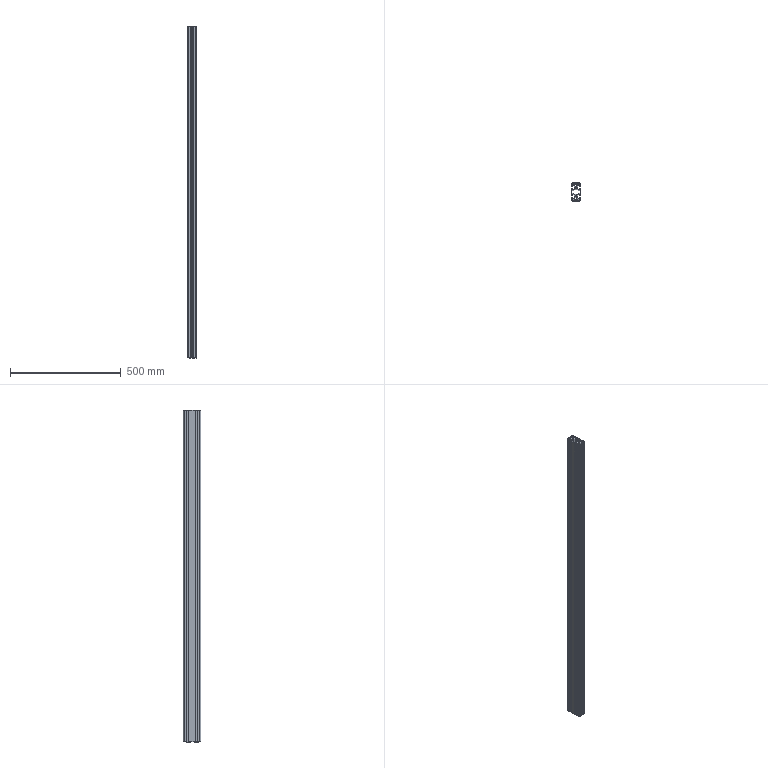Part | SolidWorks | features BaseBody 1 | 1 solid | 155 faces | box 40.002 x 80 x 1500 mm | volume 1476589 mm3 | plane 142 | cylinder 13 | commonest cylinder face diameters 9 x5 5 x4 6.8 x4